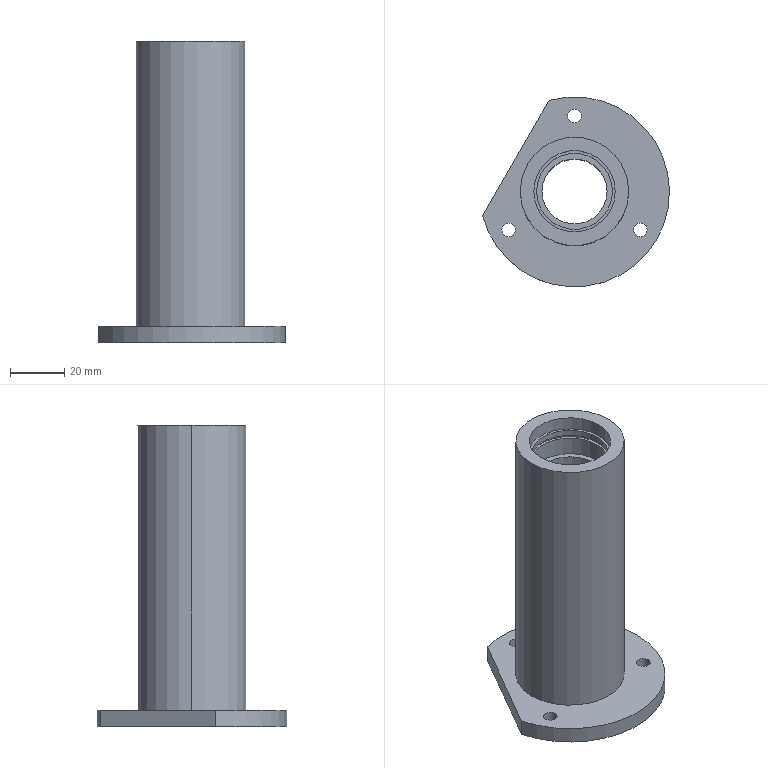Part | STEP file | Drive shaft seat SGN-5-04 | 1 solid | 42 faces | box 68.898 x 70 x 111 mm | volume 96570 mm3 | cylinder 29 | plane 13 | commonest cylinder face diameters 28 x8 5 x6 30.1 x4 24 x2 30 x2 32 x2